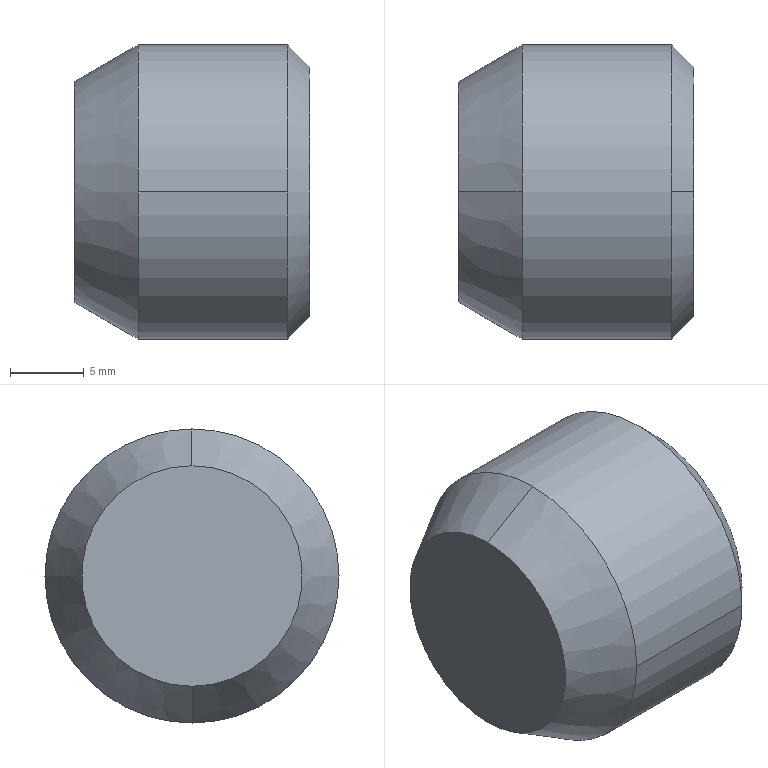Part | STEP file | Broached Hexagon Socket Set Screw - Flat Point - Metric M20x2.5 x 16 | 1 solid | 30 faces | box 16 x 20 x 20 mm | volume 3973 mm3 | plane 20 | cone 6 | cylinder 4 | commonest cylinder face diameters 10.1 x2 20 x2